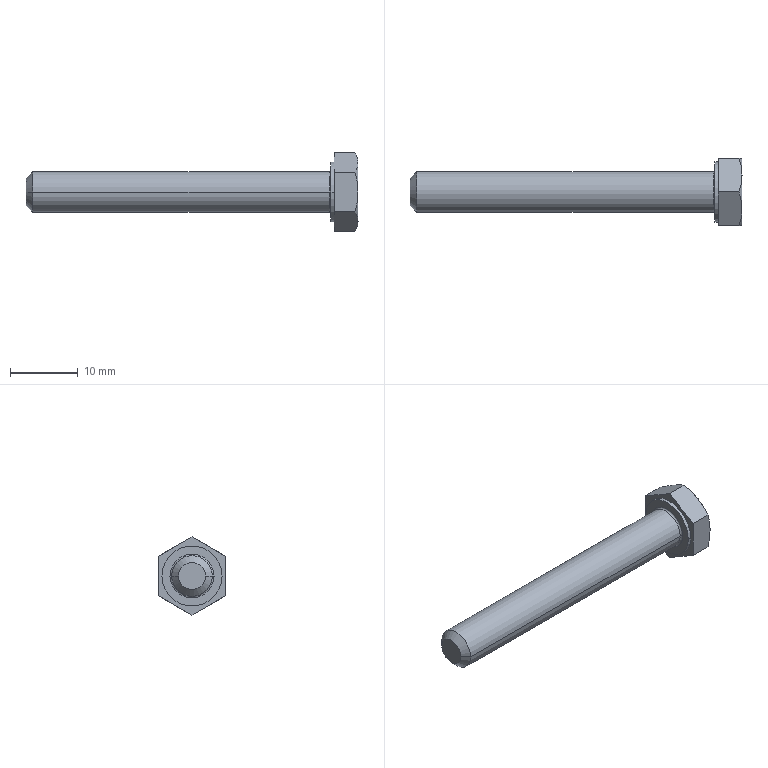Part | NX | features BREP 1 | 1 solid | 26 faces | box 49 x 10 x 11.547 mm | volume 1597 mm3 | plane 10 | cone 10 | cylinder 4 | torus 2 | commonest cylinder face diameters 6 x2 8.88 x2
STEP:
#1=CARTESIAN_POINT('',(-0.75,3.,0.));
#2=VERTEX_POINT('',#1);
#3=CARTESIAN_POINT('',(-0.75,-3.,0.));
#4=VERTEX_POINT('',#3);
#5=CARTESIAN_POINT('',(-0.75,0.,0.));
#6=DIRECTION('',(-1.,0.,0.));
#7=DIRECTION('',(0.,0.,1.));
#8=AXIS2_PLACEMENT_3D('',#5,#6,#7);
#9=CIRCLE('',#8,3.);
#10=EDGE_CURVE('',#2,#4,#9,.T.);
#11=ORIENTED_EDGE('',*,*,#10,.F.);
#12=CARTESIAN_POINT('',(-0.5,3.25,-0.000000038));
#13=VERTEX_POINT('',#12);
#14=CARTESIAN_POINT('',(-0.75,3.25,0.000000491));
#15=DIRECTION('',(0.,-0.000000151,1.));
#16=DIRECTION('',(1.,0.,0.));
#17=AXIS2_PLACEMENT_3D('',#14,#15,#16);
#18=CIRCLE('',#17,0.25);
#19=EDGE_CURVE('',#13,#2,#18,.F.);
#20=ORIENTED_EDGE('',*,*,#19,.F.);
#21=CARTESIAN_POINT('',(-0.5,-3.25,0.));
#22=VERTEX_POINT('',#21);
#23=CARTESIAN_POINT('',(-0.5,0.,0.));
#24=DIRECTION('',(-1.,0.,0.));
#25=DIRECTION('',(0.,0.,1.));
#26=AXIS2_PLACEMENT_3D('',#23,#24,#25);
#27=CIRCLE('',#26,3.25);
#28=EDGE_CURVE('',#13,#22,#27,.T.);
#29=ORIENTED_EDGE('',*,*,#28,.T.);
#30=CARTESIAN_POINT('',(-0.75,-3.25,0.));
#31=DIRECTION('',(0.,0.,-1.));
#32=DIRECTION('',(-1.,0.,0.));
#33=AXIS2_PLACEMENT_3D('',#30,#31,#32);
#34=CIRCLE('',#33,0.25);
#35=EDGE_CURVE('',#22,#4,#34,.F.);
#36=ORIENTED_EDGE('',*,*,#35,.T.);
#37=EDGE_LOOP('',(#11,#20,#29,#36));
#38=FACE_BOUND('',#37,.T.);
#39=CARTESIAN_POINT('',(-0.75,0.,0.));
#40=DIRECTION('',(-1.,0.,0.));
#41=DIRECTION('',(0.,0.998,0.06278));
#42=AXIS2_PLACEMENT_3D('',#39,#40,#41);
#43=TOROIDAL_SURFACE('',#42,3.25,0.25);
#44=ADVANCED_FACE('',(#38),#43,.F.);
#45=CARTESIAN_POINT('',(-0.75,0.,0.));
#46=DIRECTION('',(-1.,0.,0.));
#47=DIRECTION('',(0.,0.,1.));
#48=AXIS2_PLACEMENT_3D('',#45,#46,#47);
#49=CIRCLE('',#48,3.);
#50=EDGE_CURVE('',#4,#2,#49,.T.);
#51=ORIENTED_EDGE('',*,*,#50,.F.);
#52=ORIENTED_EDGE('',*,*,#35,.F.);
#53=CARTESIAN_POINT('',(-0.5,0.,0.));
#54=DIRECTION('',(-1.,0.,0.));
#55=DIRECTION('',(0.,0.,1.));
#56=AXIS2_PLACEMENT_3D('',#53,#54,#55);
#57=CIRCLE('',#56,3.25);
#58=EDGE_CURVE('',#22,#13,#57,.T.);
#59=ORIENTED_EDGE('',*,*,#58,.T.);
#60=ORIENTED_EDGE('',*,*,#19,.T.);
#61=EDGE_LOOP('',(#51,#52,#59,#60));
#62=FACE_BOUND('',#61,.T.);
#63=CARTESIAN_POINT('',(-0.75,0.,0.));
#64=DIRECTION('',(-1.,0.,0.));
#65=DIRECTION('',(0.,-1.,0.));
#66=AXIS2_PLACEMENT_3D('',#63,#64,#65);
#67=TOROIDAL_SURFACE('',#66,3.25,0.25);
#68=ADVANCED_FACE('',(#62),#67,.F.);
#69=ORIENTED_EDGE('',*,*,#28,.F.);
#70=ORIENTED_EDGE('',*,*,#58,.F.);
#71=EDGE_LOOP('',(#69,#70));
#72=FACE_BOUND('',#71,.T.);
#73=CARTESIAN_POINT('',(-0.5,-4.44,0.));
#74=VERTEX_POINT('',#73);
#75=CARTESIAN_POINT('',(-0.5,4.44,0.));
#76=VERTEX_POINT('',#75);
#77=CARTESIAN_POINT('',(-0.5,0.,0.));
#78=DIRECTION('',(-1.,0.,0.));
#79=DIRECTION('',(0.,0.,1.));
#80=AXIS2_PLACEMENT_3D('',#77,#78,#79);
#81=CIRCLE('',#80,4.44);
#82=EDGE_CURVE('',#74,#76,#81,.T.);
#83=ORIENTED_EDGE('',*,*,#82,.T.);
#84=CARTESIAN_POINT('',(-0.5,0.,0.));
#85=DIRECTION('',(-1.,0.,0.));
#86=DIRECTION('',(0.,0.,1.));
#87=AXIS2_PLACEMENT_3D('',#84,#85,#86);
#88=CIRCLE('',#87,4.44);
#89=EDGE_CURVE('',#76,#74,#88,.T.);
#90=ORIENTED_EDGE('',*,*,#89,.T.);
#91=EDGE_LOOP('',(#83,#90));
#92=FACE_BOUND('',#91,.T.);
#93=CARTESIAN_POINT('',(-0.5,0.,0.));
#94=DIRECTION('',(-1.,0.,0.));
#95=DIRECTION('',(0.,-1.,0.));
#96=AXIS2_PLACEMENT_3D('',#93,#94,#95);
#97=PLANE('',#96);
#98=ADVANCED_FACE('',(#72,#92),#97,.T.);
#99=CARTESIAN_POINT('',(-44.5,3.,0.));
#100=VERTEX_POINT('',#99);
#101=CARTESIAN_POINT('',(-22.75,3.,0.));
#102=DIRECTION('',(-1.,0.,0.));
#103=VECTOR('',#102,1000.);
#104=LINE('',#101,#103);
#105=EDGE_CURVE('',#100,#2,#104,.F.);
#106=ORIENTED_EDGE('',*,*,#105,.F.);
#107=CARTESIAN_POINT('',(-44.5,-3.,0.));
#108=VERTEX_POINT('',#107);
#109=CARTESIAN_POINT('',(-44.5,0.,0.));
#110=DIRECTION('',(-1.,0.,0.));
#111=DIRECTION('',(0.,0.,1.));
#112=AXIS2_PLACEMENT_3D('',#109,#110,#111);
#113=CIRCLE('',#112,3.);
#114=EDGE_CURVE('',#108,#100,#113,.T.);
#115=ORIENTED_EDGE('',*,*,#114,.F.);
#116=CARTESIAN_POINT('',(-22.75,-3.,0.));
#117=DIRECTION('',(-1.,0.,0.));
#118=VECTOR('',#117,1000.);
#119=LINE('',#116,#118);
#120=EDGE_CURVE('',#108,#4,#119,.F.);
#121=ORIENTED_EDGE('',*,*,#120,.T.);
#122=ORIENTED_EDGE('',*,*,#50,.T.);
#123=EDGE_LOOP('',(#106,#115,#121,#122));
#124=FACE_BOUND('',#123,.T.);
#125=CARTESIAN_POINT('',(-22.75,0.,0.));
#126=DIRECTION('',(-1.,0.,0.));
#127=DIRECTION('',(0.,-1.,0.));
#128=AXIS2_PLACEMENT_3D('',#125,#126,#127);
#129=CYLINDRICAL_SURFACE('',#128,3.);
#130=ADVANCED_FACE('',(#124),#129,.T.);
#131=ORIENTED_EDGE('',*,*,#120,.F.);
#132=CARTESIAN_POINT('',(-44.5,0.,0.));
#133=DIRECTION('',(-1.,0.,0.));
#134=DIRECTION('',(0.,0.,1.));
#135=AXIS2_PLACEMENT_3D('',#132,#133,#134);
#136=CIRCLE('',#135,3.);
#137=EDGE_CURVE('',#100,#108,#136,.T.);
#138=ORIENTED_EDGE('',*,*,#137,.F.);
#139=ORIENTED_EDGE('',*,*,#105,.T.);
#140=ORIENTED_EDGE('',*,*,#10,.T.);
#141=EDGE_LOOP('',(#131,#138,#139,#140));
#142=FACE_BOUND('',#141,.T.);
#143=CARTESIAN_POINT('',(-22.75,0.,0.));
#144=DIRECTION('',(-1.,0.,0.));
#145=DIRECTION('',(0.,-1.,0.));
#146=AXIS2_PLACEMENT_3D('',#143,#144,#145);
#147=CYLINDRICAL_SURFACE('',#146,3.);
#148=ADVANCED_FACE('',(#142),#147,.T.);
#149=CARTESIAN_POINT('',(0.,5.,-2.887));
#150=VERTEX_POINT('',#149);
#151=CARTESIAN_POINT('',(3.053,5.,-2.887));
#152=VERTEX_POINT('',#151);
#153=CARTESIAN_POINT('',(1.527,5.,-2.887));
#154=DIRECTION('',(1.,0.,0.));
#155=VECTOR('',#154,1000.);
#156=LINE('',#153,#155);
#157=EDGE_CURVE('',#150,#152,#156,.T.);
#158=ORIENTED_EDGE('',*,*,#157,.F.);
#159=CARTESIAN_POINT('',(0.,5.,2.887));
#160=VERTEX_POINT('',#159);
#161=CARTESIAN_POINT('',(0.,5.,0.));
#162=DIRECTION('',(0.,0.,1.));
#163=VECTOR('',#162,1000.);
#164=LINE('',#161,#163);
#165=EDGE_CURVE('',#150,#160,#164,.T.);
#166=ORIENTED_EDGE('',*,*,#165,.T.);
#167=CARTESIAN_POINT('',(3.053,5.,2.887));
#168=VERTEX_POINT('',#167);
#169=CARTESIAN_POINT('',(1.527,5.,2.887));
#170=DIRECTION('',(1.,0.,0.));
#171=VECTOR('',#170,1000.);
#172=LINE('',#169,#171);
#173=EDGE_CURVE('',#160,#168,#172,.T.);
#174=ORIENTED_EDGE('',*,*,#173,.T.);
#175=CARTESIAN_POINT('',(3.5,5.,0.000000051));
#176=VERTEX_POINT('',#175);
#177=CARTESIAN_POINT('',(3.053,5.,2.887));
#178=CARTESIAN_POINT('',(3.368,5.,1.798));
#179=CARTESIAN_POINT('',(3.5,5.,0.8761));
#180=CARTESIAN_POINT('',(3.5,5.,0.000000072));
#181=B_SPLINE_CURVE_WITH_KNOTS('',3,(#177,#178,#179,#180),.UNSPECIFIED.,.F.,.F.,(4,4),(0.,1.),.UNSPECIFIED.);
#182=EDGE_CURVE('',#168,#176,#181,.T.);
#183=ORIENTED_EDGE('',*,*,#182,.T.);
#184=CARTESIAN_POINT('',(3.5,5.,0.000000051));
#185=CARTESIAN_POINT('',(3.5,5.,-0.8755));
#186=CARTESIAN_POINT('',(3.368,5.,-1.797));
#187=CARTESIAN_POINT('',(3.053,5.,-2.887));
#188=B_SPLINE_CURVE_WITH_KNOTS('',3,(#184,#185,#186,#187),.UNSPECIFIED.,.F.,.F.,(4,4),(0.,1.),.UNSPECIFIED.);
#189=EDGE_CURVE('',#176,#152,#188,.T.);
#190=ORIENTED_EDGE('',*,*,#189,.T.);
#191=EDGE_LOOP('',(#158,#166,#174,#183,#190));
#192=FACE_BOUND('',#191,.T.);
#193=CARTESIAN_POINT('',(0.,5.,-2.887));
#194=DIRECTION('',(0.,1.,0.));
#195=DIRECTION('',(0.,0.,1.));
#196=AXIS2_PLACEMENT_3D('',#193,#194,#195);
#197=PLANE('',#196);
#198=ADVANCED_FACE('',(#192),#197,.T.);
#199=CARTESIAN_POINT('',(0.,0.,-5.774));
#200=VERTEX_POINT('',#199);
#201=CARTESIAN_POINT('',(3.053,0.,-5.774));
#202=VERTEX_POINT('',#201);
#203=CARTESIAN_POINT('',(1.527,0.,-5.774));
#204=DIRECTION('',(1.,0.,0.));
#205=VECTOR('',#204,1000.);
#206=LINE('',#203,#205);
#207=EDGE_CURVE('',#200,#202,#206,.T.);
#208=ORIENTED_EDGE('',*,*,#207,.F.);
#209=CARTESIAN_POINT('',(0.,2.5,-4.33));
#210=DIRECTION('',(0.,0.866,0.5));
#211=VECTOR('',#210,1000.);
#212=LINE('',#209,#211);
#213=EDGE_CURVE('',#200,#150,#212,.T.);
#214=ORIENTED_EDGE('',*,*,#213,.T.);
#215=ORIENTED_EDGE('',*,*,#157,.T.);
#216=CARTESIAN_POINT('',(3.5,2.5,-4.33));
#217=VERTEX_POINT('',#216);
#218=CARTESIAN_POINT('',(3.053,5.,-2.887));
#219=CARTESIAN_POINT('',(3.368,4.057,-3.431));
#220=CARTESIAN_POINT('',(3.5,3.259,-3.892));
#221=CARTESIAN_POINT('',(3.5,2.5,-4.33));
#222=B_SPLINE_CURVE_WITH_KNOTS('',3,(#218,#219,#220,#221),.UNSPECIFIED.,.F.,.F.,(4,4),(0.,1.),.UNSPECIFIED.);
#223=EDGE_CURVE('',#217,#152,#222,.F.);
#224=ORIENTED_EDGE('',*,*,#223,.F.);
#225=CARTESIAN_POINT('',(3.499,2.398,-4.389));
#226=VERTEX_POINT('',#225);
#227=CARTESIAN_POINT('',(3.499,2.397,-4.39));
#228=CARTESIAN_POINT('',(3.499,2.397,-4.39));
#229=CARTESIAN_POINT('',(3.499,2.397,-4.389));
#230=CARTESIAN_POINT('',(3.499,2.398,-4.389));
#231=CARTESIAN_POINT('',(3.5,2.432,-4.369));
#232=CARTESIAN_POINT('',(3.5,2.466,-4.35));
#233=CARTESIAN_POINT('',(3.5,2.5,-4.33));
#234=B_SPLINE_CURVE_WITH_KNOTS('',3,(#227,#228,#229,#230,#231,#232,#233),.UNSPECIFIED.,.F.,.F.,(4,3,4),(-0.02341,0.0002192,2.363),.PIECEWISE_BEZIER_KNOTS.);
#235=EDGE_CURVE('',#226,#217,#234,.T.);
#236=ORIENTED_EDGE('',*,*,#235,.F.);
#237=CARTESIAN_POINT('',(3.499,2.398,-4.389));
#238=CARTESIAN_POINT('',(3.488,1.671,-4.809));
#239=CARTESIAN_POINT('',(3.355,0.9034,-5.252));
#240=CARTESIAN_POINT('',(3.053,0.,-5.774));
#241=B_SPLINE_CURVE_WITH_KNOTS('',3,(#237,#238,#239,#240),.UNSPECIFIED.,.F.,.F.,(4,4),(0.,1.),.UNSPECIFIED.);
#242=EDGE_CURVE('',#226,#202,#241,.T.);
#243=ORIENTED_EDGE('',*,*,#242,.T.);
#244=EDGE_LOOP('',(#208,#214,#215,#224,#236,#243));
#245=FACE_BOUND('',#244,.T.);
#246=CARTESIAN_POINT('',(0.,0.,-5.774));
#247=DIRECTION('',(0.,0.5,-0.866));
#248=DIRECTION('',(0.,0.866,0.5));
#249=AXIS2_PLACEMENT_3D('',#246,#247,#248);
#250=PLANE('',#249);
#251=ADVANCED_FACE('',(#245),#250,.T.);
#252=CARTESIAN_POINT('',(0.,-5.,-2.887));
#253=VERTEX_POINT('',#252);
#254=CARTESIAN_POINT('',(3.053,-5.,-2.887));
#255=VERTEX_POINT('',#254);
#256=CARTESIAN_POINT('',(1.527,-5.,-2.887));
#257=DIRECTION('',(1.,0.,0.));
#258=VECTOR('',#257,1000.);
#259=LINE('',#256,#258);
#260=EDGE_CURVE('',#253,#255,#259,.T.);
#261=ORIENTED_EDGE('',*,*,#260,.F.);
#262=CARTESIAN_POINT('',(0.,-2.5,-4.33));
#263=DIRECTION('',(0.,0.866,-0.5));
#264=VECTOR('',#263,1000.);
#265=LINE('',#262,#264);
#266=EDGE_CURVE('',#253,#200,#265,.T.);
#267=ORIENTED_EDGE('',*,*,#266,.T.);
#268=ORIENTED_EDGE('',*,*,#207,.T.);
#269=CARTESIAN_POINT('',(3.5,-2.5,-4.33));
#270=VERTEX_POINT('',#269);
#271=CARTESIAN_POINT('',(3.053,0.,-5.774));
#272=CARTESIAN_POINT('',(3.368,-0.9432,-5.229));
#273=CARTESIAN_POINT('',(3.5,-1.741,-4.768));
#274=CARTESIAN_POINT('',(3.5,-2.5,-4.33));
#275=B_SPLINE_CURVE_WITH_KNOTS('',3,(#271,#272,#273,#274),.UNSPECIFIED.,.F.,.F.,(4,4),(0.,1.),.UNSPECIFIED.);
#276=EDGE_CURVE('',#202,#270,#275,.T.);
#277=ORIENTED_EDGE('',*,*,#276,.T.);
#278=CARTESIAN_POINT('',(3.5,-2.5,-4.33));
#279=CARTESIAN_POINT('',(3.5,-3.258,-3.892));
#280=CARTESIAN_POINT('',(3.368,-4.056,-3.432));
#281=CARTESIAN_POINT('',(3.053,-5.,-2.887));
#282=B_SPLINE_CURVE_WITH_KNOTS('',3,(#278,#279,#280,#281),.UNSPECIFIED.,.F.,.F.,(4,4),(0.,1.),.UNSPECIFIED.);
#283=EDGE_CURVE('',#270,#255,#282,.T.);
#284=ORIENTED_EDGE('',*,*,#283,.T.);
#285=EDGE_LOOP('',(#261,#267,#268,#277,#284));
#286=FACE_BOUND('',#285,.T.);
#287=CARTESIAN_POINT('',(0.,-5.,-2.887));
#288=DIRECTION('',(0.,-0.5,-0.866));
#289=DIRECTION('',(0.,0.866,-0.5));
#290=AXIS2_PLACEMENT_3D('',#287,#288,#289);
#291=PLANE('',#290);
#292=ADVANCED_FACE('',(#286),#291,.T.);
#293=CARTESIAN_POINT('',(0.,4.44,0.));
#294=VERTEX_POINT('',#293);
#295=CARTESIAN_POINT('',(0.,-4.44,0.));
#296=VERTEX_POINT('',#295);
#297=CARTESIAN_POINT('',(0.,0.,0.));
#298=DIRECTION('',(-1.,0.,0.));
#299=DIRECTION('',(0.,0.,1.));
#300=AXIS2_PLACEMENT_3D('',#297,#298,#299);
#301=CIRCLE('',#300,4.44);
#302=EDGE_CURVE('',#294,#296,#301,.T.);
#303=ORIENTED_EDGE('',*,*,#302,.F.);
#304=CARTESIAN_POINT('',(0.,0.,0.));
#305=DIRECTION('',(-1.,0.,0.));
#306=DIRECTION('',(0.,0.,1.));
#307=AXIS2_PLACEMENT_3D('',#304,#305,#306);
#308=CIRCLE('',#307,4.44);
#309=EDGE_CURVE('',#296,#294,#308,.T.);
#310=ORIENTED_EDGE('',*,*,#309,.F.);
#311=EDGE_LOOP('',(#303,#310));
#312=FACE_BOUND('',#311,.T.);
#313=ORIENTED_EDGE('',*,*,#213,.F.);
#314=ORIENTED_EDGE('',*,*,#266,.F.);
#315=CARTESIAN_POINT('',(0.,-5.,2.887));
#316=VERTEX_POINT('',#315);
#317=CARTESIAN_POINT('',(0.,-5.,0.));
#318=DIRECTION('',(0.,0.,-1.));
#319=VECTOR('',#318,1000.);
#320=LINE('',#317,#319);
#321=EDGE_CURVE('',#316,#253,#320,.T.);
#322=ORIENTED_EDGE('',*,*,#321,.F.);
#323=CARTESIAN_POINT('',(0.,0.,5.774));
#324=VERTEX_POINT('',#323);
#325=CARTESIAN_POINT('',(0.,-2.5,4.33));
#326=DIRECTION('',(0.,-0.866,-0.5));
#327=VECTOR('',#326,1000.);
#328=LINE('',#325,#327);
#329=EDGE_CURVE('',#324,#316,#328,.T.);
#330=ORIENTED_EDGE('',*,*,#329,.F.);
#331=CARTESIAN_POINT('',(0.,2.5,4.33));
#332=DIRECTION('',(0.,-0.866,0.5));
#333=VECTOR('',#332,1000.);
#334=LINE('',#331,#333);
#335=EDGE_CURVE('',#160,#324,#334,.T.);
#336=ORIENTED_EDGE('',*,*,#335,.F.);
#337=ORIENTED_EDGE('',*,*,#165,.F.);
#338=EDGE_LOOP('',(#313,#314,#322,#330,#336,#337));
#339=FACE_BOUND('',#338,.T.);
#340=CARTESIAN_POINT('',(0.,0.,0.));
#341=DIRECTION('',(1.,0.,0.));
#342=DIRECTION('',(0.,1.,0.));
#343=AXIS2_PLACEMENT_3D('',#340,#341,#342);
#344=PLANE('',#343);
#345=ADVANCED_FACE('',(#312,#339),#344,.F.);
#346=ORIENTED_EDGE('',*,*,#173,.F.);
#347=ORIENTED_EDGE('',*,*,#335,.T.);
#348=CARTESIAN_POINT('',(3.053,0.,5.774));
#349=VERTEX_POINT('',#348);
#350=CARTESIAN_POINT('',(1.527,0.,5.774));
#351=DIRECTION('',(1.,0.,0.));
#352=VECTOR('',#351,1000.);
#353=LINE('',#350,#352);
#354=EDGE_CURVE('',#324,#349,#353,.T.);
#355=ORIENTED_EDGE('',*,*,#354,.T.);
#356=CARTESIAN_POINT('',(3.5,2.5,4.33));
#357=VERTEX_POINT('',#356);
#358=CARTESIAN_POINT('',(3.053,0.,5.774));
#359=CARTESIAN_POINT('',(3.368,0.9432,5.229));
#360=CARTESIAN_POINT('',(3.5,1.741,4.768));
#361=CARTESIAN_POINT('',(3.5,2.5,4.33));
#362=B_SPLINE_CURVE_WITH_KNOTS('',3,(#358,#359,#360,#361),.UNSPECIFIED.,.F.,.F.,(4,4),(0.,1.),.UNSPECIFIED.);
#363=EDGE_CURVE('',#349,#357,#362,.T.);
#364=ORIENTED_EDGE('',*,*,#363,.T.);
#365=CARTESIAN_POINT('',(3.5,2.5,4.33));
#366=CARTESIAN_POINT('',(3.5,3.258,3.892));
#367=CARTESIAN_POINT('',(3.368,4.056,3.432));
#368=CARTESIAN_POINT('',(3.053,5.,2.887));
#369=B_SPLINE_CURVE_WITH_KNOTS('',3,(#365,#366,#367,#368),.UNSPECIFIED.,.F.,.F.,(4,4),(0.,1.),.UNSPECIFIED.);
#370=EDGE_CURVE('',#357,#168,#369,.T.);
#371=ORIENTED_EDGE('',*,*,#370,.T.);
#372=EDGE_LOOP('',(#346,#347,#355,#364,#371));
#373=FACE_BOUND('',#372,.T.);
#374=CARTESIAN_POINT('',(0.,5.,2.887));
#375=DIRECTION('',(0.,0.5,0.866));
#376=DIRECTION('',(0.,-0.866,0.5));
#377=AXIS2_PLACEMENT_3D('',#374,#375,#376);
#378=PLANE('',#377);
#379=ADVANCED_FACE('',(#373),#378,.T.);
#380=ORIENTED_EDGE('',*,*,#370,.F.);
#381=CARTESIAN_POINT('',(3.5,0.,0.));
#382=DIRECTION('',(1.,0.,0.));
#383=DIRECTION('',(0.,0.,-1.));
#384=AXIS2_PLACEMENT_3D('',#381,#382,#383);
#385=CIRCLE('',#384,5.);
#386=EDGE_CURVE('',#176,#357,#385,.T.);
#387=ORIENTED_EDGE('',*,*,#386,.F.);
#388=ORIENTED_EDGE('',*,*,#182,.F.);
#389=EDGE_LOOP('',(#380,#387,#388));
#390=FACE_BOUND('',#389,.T.);
#391=CARTESIAN_POINT('',(3.5,0.,0.));
#392=DIRECTION('',(-1.,0.,0.));
#393=DIRECTION('',(0.,-0.4794,0.8776));
#394=AXIS2_PLACEMENT_3D('',#391,#392,#393);
#395=CONICAL_SURFACE('',#394,5.,1.047);
#396=ADVANCED_FACE('',(#390),#395,.T.);
#397=CARTESIAN_POINT('',(3.5,0.,0.));
#398=DIRECTION('',(1.,0.,0.));
#399=DIRECTION('',(0.,0.,-1.));
#400=AXIS2_PLACEMENT_3D('',#397,#398,#399);
#401=CIRCLE('',#400,5.);
#402=EDGE_CURVE('',#217,#176,#401,.T.);
#403=ORIENTED_EDGE('',*,*,#402,.F.);
#404=ORIENTED_EDGE('',*,*,#223,.T.);
#405=ORIENTED_EDGE('',*,*,#189,.F.);
#406=EDGE_LOOP('',(#403,#404,#405));
#407=FACE_BOUND('',#406,.T.);
#408=CARTESIAN_POINT('',(3.5,0.,0.));
#409=DIRECTION('',(-1.,0.,0.));
#410=DIRECTION('',(0.,-0.4794,0.8776));
#411=AXIS2_PLACEMENT_3D('',#408,#409,#410);
#412=CONICAL_SURFACE('',#411,5.,1.047);
#413=ADVANCED_FACE('',(#407),#412,.T.);
#414=CARTESIAN_POINT('',(3.5,2.397,-4.388));
#415=VERTEX_POINT('',#414);
#416=CARTESIAN_POINT('',(3.5,0.,0.));
#417=DIRECTION('',(1.,0.,0.));
#418=DIRECTION('',(0.,0.,-1.));
#419=AXIS2_PLACEMENT_3D('',#416,#417,#418);
#420=CIRCLE('',#419,5.);
#421=EDGE_CURVE('',#415,#217,#420,.T.);
#422=ORIENTED_EDGE('',*,*,#421,.F.);
#423=CARTESIAN_POINT('',(3.277,2.583,-4.727));
#424=DIRECTION('',(-0.5,0.4152,-0.76));
#425=VECTOR('',#424,1000.);
#426=LINE('',#423,#425);
#427=EDGE_CURVE('',#415,#226,#426,.T.);
#428=ORIENTED_EDGE('',*,*,#427,.T.);
#429=ORIENTED_EDGE('',*,*,#235,.T.);
#430=EDGE_LOOP('',(#422,#428,#429));
#431=FACE_BOUND('',#430,.T.);
#432=CARTESIAN_POINT('',(3.5,0.,0.));
#433=DIRECTION('',(-1.,0.,0.));
#434=DIRECTION('',(0.,-0.4794,0.8776));
#435=AXIS2_PLACEMENT_3D('',#432,#433,#434);
#436=CONICAL_SURFACE('',#435,5.,1.047);
#437=ADVANCED_FACE('',(#431),#436,.T.);
#438=ORIENTED_EDGE('',*,*,#242,.F.);
#439=ORIENTED_EDGE('',*,*,#427,.F.);
#440=CARTESIAN_POINT('',(3.5,0.,0.));
#441=DIRECTION('',(1.,0.,0.));
#442=DIRECTION('',(0.,0.,-1.));
#443=AXIS2_PLACEMENT_3D('',#440,#441,#442);
#444=CIRCLE('',#443,5.);
#445=EDGE_CURVE('',#270,#415,#444,.T.);
#446=ORIENTED_EDGE('',*,*,#445,.F.);
#447=ORIENTED_EDGE('',*,*,#276,.F.);
#448=EDGE_LOOP('',(#438,#439,#446,#447));
#449=FACE_BOUND('',#448,.T.);
#450=CARTESIAN_POINT('',(3.5,0.,0.));
#451=DIRECTION('',(-1.,0.,0.));
#452=DIRECTION('',(0.,-0.4794,0.8776));
#453=AXIS2_PLACEMENT_3D('',#450,#451,#452);
#454=CONICAL_SURFACE('',#453,5.,1.047);
#455=ADVANCED_FACE('',(#449),#454,.T.);
#456=ORIENTED_EDGE('',*,*,#283,.F.);
#457=CARTESIAN_POINT('',(3.5,-5.,-0.000000051));
#458=VERTEX_POINT('',#457);
#459=CARTESIAN_POINT('',(3.5,0.,0.));
#460=DIRECTION('',(1.,0.,0.));
#461=DIRECTION('',(0.,0.,-1.));
#462=AXIS2_PLACEMENT_3D('',#459,#460,#461);
#463=CIRCLE('',#462,5.);
#464=EDGE_CURVE('',#458,#270,#463,.T.);
#465=ORIENTED_EDGE('',*,*,#464,.F.);
#466=CARTESIAN_POINT('',(3.053,-5.,-2.887));
#467=CARTESIAN_POINT('',(3.167,-5.,-2.495));
#468=CARTESIAN_POINT('',(3.256,-5.,-2.136));
#469=CARTESIAN_POINT('',(3.327,-5.,-1.799));
#470=CARTESIAN_POINT('',(3.424,-5.,-1.228));
#471=CARTESIAN_POINT('',(3.477,-5.,-0.69));
#472=CARTESIAN_POINT('',(3.492,-5.,-0.4586));
#473=CARTESIAN_POINT('',(3.5,-5.,-0.2293));
#474=CARTESIAN_POINT('',(3.5,-5.,-0.000000051));
#475=B_SPLINE_CURVE_WITH_KNOTS('',5,(#466,#467,#468,#469,#470,#471,#472,#473,#474),.UNSPECIFIED.,.F.,.F.,(6,3,6),(0.,29.491,52.477),.UNSPECIFIED.);
#476=EDGE_CURVE('',#255,#458,#475,.T.);
#477=ORIENTED_EDGE('',*,*,#476,.F.);
#478=EDGE_LOOP('',(#456,#465,#477));
#479=FACE_BOUND('',#478,.T.);
#480=CARTESIAN_POINT('',(3.5,0.,0.));
#481=DIRECTION('',(-1.,0.,0.));
#482=DIRECTION('',(0.,-0.4794,0.8776));
#483=AXIS2_PLACEMENT_3D('',#480,#481,#482);
#484=CONICAL_SURFACE('',#483,5.,1.047);
#485=ADVANCED_FACE('',(#479),#484,.T.);
#486=CARTESIAN_POINT('',(3.5,-2.397,4.388));
#487=VERTEX_POINT('',#486);
#488=CARTESIAN_POINT('',(3.5,-2.5,4.33));
#489=VERTEX_POINT('',#488);
#490=CARTESIAN_POINT('',(3.5,0.,0.));
#491=DIRECTION('',(1.,0.,0.));
#492=DIRECTION('',(0.,0.,-1.));
#493=AXIS2_PLACEMENT_3D('',#490,#491,#492);
#494=CIRCLE('',#493,5.);
#495=EDGE_CURVE('',#487,#489,#494,.T.);
#496=ORIENTED_EDGE('',*,*,#495,.F.);
#497=CARTESIAN_POINT('',(3.5,-2.398,4.389));
#498=VERTEX_POINT('',#497);
#499=CARTESIAN_POINT('',(3.277,-2.583,4.727));
#500=DIRECTION('',(-0.5,-0.4152,0.76));
#501=VECTOR('',#500,1000.);
#502=LINE('',#499,#501);
#503=EDGE_CURVE('',#487,#498,#502,.T.);
#504=ORIENTED_EDGE('',*,*,#503,.T.);
#505=CARTESIAN_POINT('',(3.5,-2.5,4.33));
#506=CARTESIAN_POINT('',(3.5,-2.466,4.35));
#507=CARTESIAN_POINT('',(3.5,-2.432,4.369));
#508=CARTESIAN_POINT('',(3.5,-2.398,4.389));
#509=B_SPLINE_CURVE_WITH_KNOTS('',3,(#505,#506,#507,#508),.UNSPECIFIED.,.F.,.F.,(4,4),(0.,1.),.UNSPECIFIED.);
#510=EDGE_CURVE('',#498,#489,#509,.F.);
#511=ORIENTED_EDGE('',*,*,#510,.T.);
#512=EDGE_LOOP('',(#496,#504,#511));
#513=FACE_BOUND('',#512,.T.);
#514=CARTESIAN_POINT('',(3.5,0.,0.));
#515=DIRECTION('',(-1.,0.,0.));
#516=DIRECTION('',(0.,-0.4794,0.8776));
#517=AXIS2_PLACEMENT_3D('',#514,#515,#516);
#518=CONICAL_SURFACE('',#517,5.,1.047);
#519=ADVANCED_FACE('',(#513),#518,.T.);
#520=CARTESIAN_POINT('',(3.5,-2.419,4.377));
#521=CARTESIAN_POINT('',(3.499,-2.415,4.379));
#522=CARTESIAN_POINT('',(3.499,-2.411,4.382));
#523=CARTESIAN_POINT('',(3.499,-2.406,4.384));
#524=CARTESIAN_POINT('',(3.499,-2.402,4.387));
#525=CARTESIAN_POINT('',(3.499,-2.398,4.389));
#526=CARTESIAN_POINT('',(3.494,-2.077,4.574));
#527=CARTESIAN_POINT('',(3.469,-1.755,4.76));
#528=CARTESIAN_POINT('',(3.424,-1.425,4.951));
#529=CARTESIAN_POINT('',(3.334,-0.9564,5.221));
#530=CARTESIAN_POINT('',(3.19,-0.4353,5.522));
#531=CARTESIAN_POINT('',(3.149,-0.2952,5.603));
#532=CARTESIAN_POINT('',(3.104,-0.1504,5.687));
#533=CARTESIAN_POINT('',(3.053,0.,5.774));
#534=B_SPLINE_CURVE_WITH_KNOTS('',5,(#520,#521,#522,#523,#524,#525,#526,#527,#528,#529,#530,#531,#532,#533),.UNSPECIFIED.,.F.,.F.,(6,5,3,6),(-0.5011,0.,37.038,50.105),.UNSPECIFIED.);
#535=EDGE_CURVE('',#498,#349,#534,.T.);
#536=ORIENTED_EDGE('',*,*,#535,.F.);
#537=ORIENTED_EDGE('',*,*,#503,.F.);
#538=CARTESIAN_POINT('',(3.5,0.,0.));
#539=DIRECTION('',(1.,0.,0.));
#540=DIRECTION('',(0.,0.,-1.));
#541=AXIS2_PLACEMENT_3D('',#538,#539,#540);
#542=CIRCLE('',#541,5.);
#543=EDGE_CURVE('',#357,#487,#542,.T.);
#544=ORIENTED_EDGE('',*,*,#543,.F.);
#545=ORIENTED_EDGE('',*,*,#363,.F.);
#546=EDGE_LOOP('',(#536,#537,#544,#545));
#547=FACE_BOUND('',#546,.T.);
#548=CARTESIAN_POINT('',(3.5,0.,0.));
#549=DIRECTION('',(-1.,0.,0.));
#550=DIRECTION('',(0.,-0.4794,0.8776));
#551=AXIS2_PLACEMENT_3D('',#548,#549,#550);
#552=CONICAL_SURFACE('',#551,5.,1.047);
#553=ADVANCED_FACE('',(#547),#552,.T.);
#554=CARTESIAN_POINT('',(3.053,-5.,2.887));
#555=VERTEX_POINT('',#554);
#556=CARTESIAN_POINT('',(1.527,-5.,2.887));
#557=DIRECTION('',(1.,0.,0.));
#558=VECTOR('',#557,1000.);
#559=LINE('',#556,#558);
#560=EDGE_CURVE('',#316,#555,#559,.T.);
#561=ORIENTED_EDGE('',*,*,#560,.F.);
#562=ORIENTED_EDGE('',*,*,#321,.T.);
#563=ORIENTED_EDGE('',*,*,#260,.T.);
#564=ORIENTED_EDGE('',*,*,#476,.T.);
#565=CARTESIAN_POINT('',(3.5,-5.,-0.000000051));
#566=CARTESIAN_POINT('',(3.5,-5.,0.8755));
#567=CARTESIAN_POINT('',(3.368,-5.,1.797));
#568=CARTESIAN_POINT('',(3.053,-5.,2.887));
#569=B_SPLINE_CURVE_WITH_KNOTS('',3,(#565,#566,#567,#568),.UNSPECIFIED.,.F.,.F.,(4,4),(0.,1.),.UNSPECIFIED.);
#570=EDGE_CURVE('',#458,#555,#569,.T.);
#571=ORIENTED_EDGE('',*,*,#570,.T.);
#572=EDGE_LOOP('',(#561,#562,#563,#564,#571));
#573=FACE_BOUND('',#572,.T.);
#574=CARTESIAN_POINT('',(0.,-5.,2.887));
#575=DIRECTION('',(0.,-1.,0.));
#576=DIRECTION('',(0.,0.,-1.));
#577=AXIS2_PLACEMENT_3D('',#574,#575,#576);
#578=PLANE('',#577);
#579=ADVANCED_FACE('',(#573),#578,.T.);
#580=ORIENTED_EDGE('',*,*,#354,.F.);
#581=ORIENTED_EDGE('',*,*,#329,.T.);
#582=ORIENTED_EDGE('',*,*,#560,.T.);
#583=CARTESIAN_POINT('',(3.053,-5.,2.887));
#584=CARTESIAN_POINT('',(3.368,-4.057,3.431));
#585=CARTESIAN_POINT('',(3.5,-3.259,3.892));
#586=CARTESIAN_POINT('',(3.5,-2.5,4.33));
#587=B_SPLINE_CURVE_WITH_KNOTS('',3,(#583,#584,#585,#586),.UNSPECIFIED.,.F.,.F.,(4,4),(0.,1.),.UNSPECIFIED.);
#588=EDGE_CURVE('',#489,#555,#587,.F.);
#589=ORIENTED_EDGE('',*,*,#588,.F.);
#590=ORIENTED_EDGE('',*,*,#510,.F.);
#591=ORIENTED_EDGE('',*,*,#535,.T.);
#592=EDGE_LOOP('',(#580,#581,#582,#589,#590,#591));
#593=FACE_BOUND('',#592,.T.);
#594=CARTESIAN_POINT('',(0.,0.,5.774));
#595=DIRECTION('',(0.,-0.5,0.866));
#596=DIRECTION('',(0.,-0.866,-0.5));
#597=AXIS2_PLACEMENT_3D('',#594,#595,#596);
#598=PLANE('',#597);
#599=ADVANCED_FACE('',(#593),#598,.T.);
#600=ORIENTED_EDGE('',*,*,#543,.T.);
#601=ORIENTED_EDGE('',*,*,#495,.T.);
#602=CARTESIAN_POINT('',(3.5,0.,0.));
#603=DIRECTION('',(-1.,0.,0.));
#604=DIRECTION('',(0.,0.,1.));
#605=AXIS2_PLACEMENT_3D('',#602,#603,#604);
#606=CIRCLE('',#605,5.);
#607=EDGE_CURVE('',#458,#489,#606,.T.);
#608=ORIENTED_EDGE('',*,*,#607,.F.);
#609=ORIENTED_EDGE('',*,*,#464,.T.);
#610=ORIENTED_EDGE('',*,*,#445,.T.);
#611=ORIENTED_EDGE('',*,*,#421,.T.);
#612=ORIENTED_EDGE('',*,*,#402,.T.);
#613=ORIENTED_EDGE('',*,*,#386,.T.);
#614=EDGE_LOOP('',(#600,#601,#608,#609,#610,#611,#612,#613));
#615=FACE_BOUND('',#614,.T.);
#616=CARTESIAN_POINT('',(3.5,0.,0.));
#617=DIRECTION('',(1.,0.,0.));
#618=DIRECTION('',(0.,1.,0.));
#619=AXIS2_PLACEMENT_3D('',#616,#617,#618);
#620=PLANE('',#619);
#621=ADVANCED_FACE('',(#615),#620,.T.);
#622=ORIENTED_EDGE('',*,*,#607,.T.);
#623=ORIENTED_EDGE('',*,*,#588,.T.);
#624=ORIENTED_EDGE('',*,*,#570,.F.);
#625=EDGE_LOOP('',(#622,#623,#624));
#626=FACE_BOUND('',#625,.T.);
#627=CARTESIAN_POINT('',(3.5,0.,0.));
#628=DIRECTION('',(-1.,0.,0.));
#629=DIRECTION('',(0.,-0.4794,0.8776));
#630=AXIS2_PLACEMENT_3D('',#627,#628,#629);
#631=CONICAL_SURFACE('',#630,5.,1.047);
#632=ADVANCED_FACE('',(#626),#631,.T.);
#633=CARTESIAN_POINT('',(-0.25,4.44,0.));
#634=DIRECTION('',(-1.,0.,0.));
#635=VECTOR('',#634,1000.);
#636=LINE('',#633,#635);
#637=EDGE_CURVE('',#76,#294,#636,.F.);
#638=ORIENTED_EDGE('',*,*,#637,.T.);
#639=ORIENTED_EDGE('',*,*,#302,.T.);
#640=CARTESIAN_POINT('',(-0.25,-4.44,0.));
#641=DIRECTION('',(-1.,0.,0.));
#642=VECTOR('',#641,1000.);
#643=LINE('',#640,#642);
#644=EDGE_CURVE('',#74,#296,#643,.F.);
#645=ORIENTED_EDGE('',*,*,#644,.F.);
#646=ORIENTED_EDGE('',*,*,#89,.F.);
#647=EDGE_LOOP('',(#638,#639,#645,#646));
#648=FACE_BOUND('',#647,.T.);
#649=CARTESIAN_POINT('',(-0.25,0.,0.));
#650=DIRECTION('',(-1.,0.,0.));
#651=DIRECTION('',(0.,-1.,0.));
#652=AXIS2_PLACEMENT_3D('',#649,#650,#651);
#653=CYLINDRICAL_SURFACE('',#652,4.44);
#654=ADVANCED_FACE('',(#648),#653,.T.);
#655=ORIENTED_EDGE('',*,*,#644,.T.);
#656=ORIENTED_EDGE('',*,*,#309,.T.);
#657=ORIENTED_EDGE('',*,*,#637,.F.);
#658=ORIENTED_EDGE('',*,*,#82,.F.);
#659=EDGE_LOOP('',(#655,#656,#657,#658));
#660=FACE_BOUND('',#659,.T.);
#661=CARTESIAN_POINT('',(-0.25,0.,0.));
#662=DIRECTION('',(-1.,0.,0.));
#663=DIRECTION('',(0.,-1.,0.));
#664=AXIS2_PLACEMENT_3D('',#661,#662,#663);
#665=CYLINDRICAL_SURFACE('',#664,4.44);
#666=ADVANCED_FACE('',(#660),#665,.T.);
#667=CARTESIAN_POINT('',(-45.5,-2.,0.));
#668=VERTEX_POINT('',#667);
#669=CARTESIAN_POINT('',(-45.,-2.5,0.));
#670=DIRECTION('',(0.7071,-0.7071,0.));
#671=VECTOR('',#670,1000.);
#672=LINE('',#669,#671);
#673=EDGE_CURVE('',#668,#108,#672,.T.);
#674=ORIENTED_EDGE('',*,*,#673,.T.);
#675=ORIENTED_EDGE('',*,*,#114,.T.);
#676=CARTESIAN_POINT('',(-45.5,2.,-0.000000315));
#677=VERTEX_POINT('',#676);
#678=CARTESIAN_POINT('',(-45.,2.5,0.));
#679=DIRECTION('',(0.7071,0.7071,0.));
#680=VECTOR('',#679,1000.);
#681=LINE('',#678,#680);
#682=EDGE_CURVE('',#677,#100,#681,.T.);
#683=ORIENTED_EDGE('',*,*,#682,.F.);
#684=CARTESIAN_POINT('',(-45.5,0.,0.));
#685=DIRECTION('',(-1.,0.,0.));
#686=DIRECTION('',(0.,0.,1.));
#687=AXIS2_PLACEMENT_3D('',#684,#685,#686);
#688=CIRCLE('',#687,2.);
#689=EDGE_CURVE('',#668,#677,#688,.T.);
#690=ORIENTED_EDGE('',*,*,#689,.F.);
#691=EDGE_LOOP('',(#674,#675,#683,#690));
#692=FACE_BOUND('',#691,.T.);
#693=CARTESIAN_POINT('',(-47.5,0.,0.));
#694=DIRECTION('',(1.,0.,0.));
#695=DIRECTION('',(0.,-1.,0.));
#696=AXIS2_PLACEMENT_3D('',#693,#694,#695);
#697=CONICAL_SURFACE('',#696,0.,0.7854);
#698=ADVANCED_FACE('',(#692),#697,.T.);
#699=ORIENTED_EDGE('',*,*,#682,.T.);
#700=ORIENTED_EDGE('',*,*,#137,.T.);
#701=ORIENTED_EDGE('',*,*,#673,.F.);
#702=CARTESIAN_POINT('',(-45.5,0.,0.));
#703=DIRECTION('',(-1.,0.,0.));
#704=DIRECTION('',(0.,0.,1.));
#705=AXIS2_PLACEMENT_3D('',#702,#703,#704);
#706=CIRCLE('',#705,2.);
#707=EDGE_CURVE('',#677,#668,#706,.T.);
#708=ORIENTED_EDGE('',*,*,#707,.F.);
#709=EDGE_LOOP('',(#699,#700,#701,#708));
#710=FACE_BOUND('',#709,.T.);
#711=CARTESIAN_POINT('',(-47.5,0.,0.));
#712=DIRECTION('',(1.,0.,0.));
#713=DIRECTION('',(0.,0.941,0.3385));
#714=AXIS2_PLACEMENT_3D('',#711,#712,#713);
#715=CONICAL_SURFACE('',#714,0.,0.7854);
#716=ADVANCED_FACE('',(#710),#715,.T.);
#717=ORIENTED_EDGE('',*,*,#707,.T.);
#718=ORIENTED_EDGE('',*,*,#689,.T.);
#719=EDGE_LOOP('',(#717,#718));
#720=FACE_BOUND('',#719,.T.);
#721=CARTESIAN_POINT('',(-45.5,0.,0.));
#722=DIRECTION('',(-1.,0.,0.));
#723=DIRECTION('',(0.,-1.,0.));
#724=AXIS2_PLACEMENT_3D('',#721,#722,#723);
#725=PLANE('',#724);
#726=ADVANCED_FACE('',(#720),#725,.T.);
#727=CLOSED_SHELL('',(#44,#68,#98,#130,#148,#198,#251,#292,#345,#379,#396,#413,#437,#455,#485,#519,#553,#579,#599,#621,#632,#654,#666,#698,#716,#726));
#728=MANIFOLD_SOLID_BREP('',#727);
#729=(LENGTH_UNIT()NAMED_UNIT(*)SI_UNIT(.MILLI.,.METRE.));
#730=UNCERTAINTY_MEASURE_WITH_UNIT(LENGTH_MEASURE(0.0508),#729,'','');
#731=(NAMED_UNIT(*)PLANE_ANGLE_UNIT()SI_UNIT($,.RADIAN.));
#732=(NAMED_UNIT(*)SI_UNIT($,.STERADIAN.)SOLID_ANGLE_UNIT());
#733=(GEOMETRIC_REPRESENTATION_CONTEXT(3)GLOBAL_UNCERTAINTY_ASSIGNED_CONTEXT((#730))GLOBAL_UNIT_ASSIGNED_CONTEXT((#729,#731,#732))REPRESENTATION_CONTEXT('',''));
#734=ADVANCED_BREP_SHAPE_REPRESENTATION('',(#728),#733);